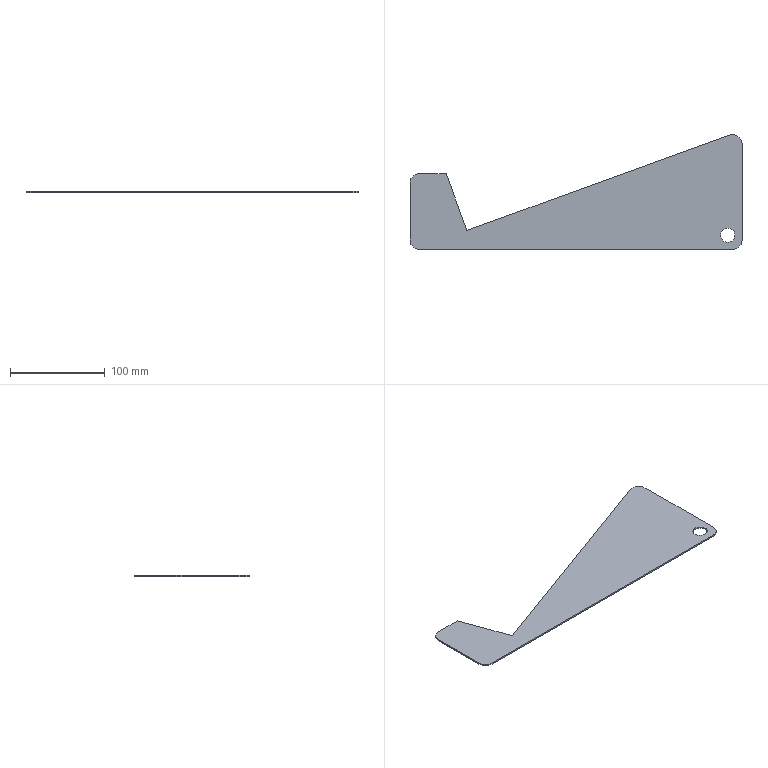Part | SolidWorks | features FlatPattern 1, SMBaseFlange 1, SheetMetal 1 | 1 solid | 14 faces | box 350 x 121.27 x 1.6 mm | volume 39939 mm3 | plane 8 | cylinder 6 | commonest cylinder face diameters 20 x4 15 x2
STEP:
#1=CARTESIAN_POINT('',(633.,10.,1.6));
#2=VERTEX_POINT('',#1);
#3=CARTESIAN_POINT('',(648.,10.,1.6));
#4=VERTEX_POINT('',#3);
#5=CARTESIAN_POINT('',(640.5,10.,1.6));
#6=DIRECTION('',(0.,0.,1.));
#7=DIRECTION('',(1.,0.,0.));
#8=AXIS2_PLACEMENT_3D('',#5,#6,#7);
#9=CIRCLE('',#8,7.5);
#10=EDGE_CURVE('',#2,#4,#9,.T.);
#11=ORIENTED_EDGE('',*,*,#10,.T.);
#12=CARTESIAN_POINT('',(648.,10.,0.));
#13=VERTEX_POINT('',#12);
#14=CARTESIAN_POINT('',(648.,10.,1.6));
#15=DIRECTION('',(0.,0.,-1.));
#16=VECTOR('',#15,1000.);
#17=LINE('',#14,#16);
#18=EDGE_CURVE('',#4,#13,#17,.T.);
#19=ORIENTED_EDGE('',*,*,#18,.T.);
#20=CARTESIAN_POINT('',(633.,10.,0.));
#21=VERTEX_POINT('',#20);
#22=CARTESIAN_POINT('',(640.5,10.,0.));
#23=DIRECTION('',(0.,0.,1.));
#24=DIRECTION('',(1.,0.,0.));
#25=AXIS2_PLACEMENT_3D('',#22,#23,#24);
#26=CIRCLE('',#25,7.5);
#27=EDGE_CURVE('',#21,#13,#26,.T.);
#28=ORIENTED_EDGE('',*,*,#27,.F.);
#29=CARTESIAN_POINT('',(633.,10.,1.6));
#30=DIRECTION('',(0.,0.,-1.));
#31=VECTOR('',#30,1000.);
#32=LINE('',#29,#31);
#33=EDGE_CURVE('',#2,#21,#32,.T.);
#34=ORIENTED_EDGE('',*,*,#33,.F.);
#35=EDGE_LOOP('',(#11,#19,#28,#34));
#36=FACE_OUTER_BOUND('',#35,.T.);
#37=CARTESIAN_POINT('',(640.5,10.,1.6));
#38=DIRECTION('',(0.,0.,-1.));
#39=DIRECTION('',(-1.,0.,0.));
#40=AXIS2_PLACEMENT_3D('',#37,#38,#39);
#41=CYLINDRICAL_SURFACE('',#40,7.5);
#42=ADVANCED_FACE('',(#36),#41,.F.);
#43=CARTESIAN_POINT('',(343.662,75.,1.6));
#44=VERTEX_POINT('',#43);
#45=CARTESIAN_POINT('',(315.5,75.,1.6));
#46=VERTEX_POINT('',#45);
#47=CARTESIAN_POINT('',(343.662,75.,1.6));
#48=DIRECTION('',(-1.,0.,0.));
#49=VECTOR('',#48,1000.);
#50=LINE('',#47,#49);
#51=EDGE_CURVE('',#44,#46,#50,.T.);
#52=ORIENTED_EDGE('',*,*,#51,.T.);
#53=CARTESIAN_POINT('',(305.5,65.,1.6));
#54=VERTEX_POINT('',#53);
#55=CARTESIAN_POINT('',(315.5,65.,1.6));
#56=DIRECTION('',(0.,0.,1.));
#57=DIRECTION('',(1.,0.,0.));
#58=AXIS2_PLACEMENT_3D('',#55,#56,#57);
#59=CIRCLE('',#58,10.);
#60=EDGE_CURVE('',#46,#54,#59,.T.);
#61=ORIENTED_EDGE('',*,*,#60,.T.);
#62=CARTESIAN_POINT('',(305.5,5.,1.6));
#63=VERTEX_POINT('',#62);
#64=CARTESIAN_POINT('',(305.5,5.,1.6));
#65=DIRECTION('',(0.,-1.,0.));
#66=VECTOR('',#65,1000.);
#67=LINE('',#64,#66);
#68=EDGE_CURVE('',#54,#63,#67,.T.);
#69=ORIENTED_EDGE('',*,*,#68,.T.);
#70=CARTESIAN_POINT('',(315.5,-5.,1.6));
#71=VERTEX_POINT('',#70);
#72=CARTESIAN_POINT('',(315.5,5.,1.6));
#73=DIRECTION('',(0.,0.,1.));
#74=DIRECTION('',(-1.,0.,0.));
#75=AXIS2_PLACEMENT_3D('',#72,#73,#74);
#76=CIRCLE('',#75,10.);
#77=EDGE_CURVE('',#63,#71,#76,.T.);
#78=ORIENTED_EDGE('',*,*,#77,.T.);
#79=CARTESIAN_POINT('',(645.5,-5.,1.6));
#80=VERTEX_POINT('',#79);
#81=CARTESIAN_POINT('',(645.5,-5.,1.6));
#82=DIRECTION('',(1.,0.,0.));
#83=VECTOR('',#82,1000.);
#84=LINE('',#81,#83);
#85=EDGE_CURVE('',#71,#80,#84,.T.);
#86=ORIENTED_EDGE('',*,*,#85,.T.);
#87=CARTESIAN_POINT('',(655.5,5.,1.6));
#88=VERTEX_POINT('',#87);
#89=CARTESIAN_POINT('',(645.5,5.,1.6));
#90=DIRECTION('',(0.,0.,1.));
#91=DIRECTION('',(-1.,0.,0.));
#92=AXIS2_PLACEMENT_3D('',#89,#90,#91);
#93=CIRCLE('',#92,10.);
#94=EDGE_CURVE('',#80,#88,#93,.T.);
#95=ORIENTED_EDGE('',*,*,#94,.T.);
#96=CARTESIAN_POINT('',(655.5,106.27,1.6));
#97=VERTEX_POINT('',#96);
#98=CARTESIAN_POINT('',(655.5,106.27,1.6));
#99=DIRECTION('',(0.,1.,0.));
#100=VECTOR('',#99,1000.);
#101=LINE('',#98,#100);
#102=EDGE_CURVE('',#88,#97,#101,.T.);
#103=ORIENTED_EDGE('',*,*,#102,.T.);
#104=CARTESIAN_POINT('',(642.08,115.667,1.6));
#105=VERTEX_POINT('',#104);
#106=CARTESIAN_POINT('',(645.5,106.27,1.6));
#107=DIRECTION('',(0.,0.,1.));
#108=DIRECTION('',(-1.,0.,0.));
#109=AXIS2_PLACEMENT_3D('',#106,#107,#108);
#110=CIRCLE('',#109,10.);
#111=EDGE_CURVE('',#97,#105,#110,.T.);
#112=ORIENTED_EDGE('',*,*,#111,.T.);
#113=CARTESIAN_POINT('',(365.5,15.,1.6));
#114=VERTEX_POINT('',#113);
#115=CARTESIAN_POINT('',(365.5,15.,1.6));
#116=DIRECTION('',(-0.9397,-0.342,0.));
#117=VECTOR('',#116,1000.);
#118=LINE('',#115,#117);
#119=EDGE_CURVE('',#105,#114,#118,.T.);
#120=ORIENTED_EDGE('',*,*,#119,.T.);
#121=CARTESIAN_POINT('',(365.5,15.,1.6));
#122=DIRECTION('',(-0.342,0.9397,0.));
#123=VECTOR('',#122,1000.);
#124=LINE('',#121,#123);
#125=EDGE_CURVE('',#114,#44,#124,.T.);
#126=ORIENTED_EDGE('',*,*,#125,.T.);
#127=EDGE_LOOP('',(#52,#61,#69,#78,#86,#95,#103,#112,#120,#126));
#128=FACE_OUTER_BOUND('',#127,.T.);
#129=ORIENTED_EDGE('',*,*,#10,.F.);
#130=CARTESIAN_POINT('',(640.5,10.,1.6));
#131=DIRECTION('',(0.,0.,1.));
#132=DIRECTION('',(1.,0.,0.));
#133=AXIS2_PLACEMENT_3D('',#130,#131,#132);
#134=CIRCLE('',#133,7.5);
#135=EDGE_CURVE('',#4,#2,#134,.T.);
#136=ORIENTED_EDGE('',*,*,#135,.F.);
#137=EDGE_LOOP('',(#129,#136));
#138=FACE_BOUND('',#137,.T.);
#139=CARTESIAN_POINT('',(315.5,65.,1.6));
#140=DIRECTION('',(0.,0.,1.));
#141=DIRECTION('',(1.,0.,0.));
#142=AXIS2_PLACEMENT_3D('',#139,#140,#141);
#143=PLANE('',#142);
#144=ADVANCED_FACE('',(#128,#138),#143,.T.);
#145=CARTESIAN_POINT('',(343.662,75.,0.));
#146=VERTEX_POINT('',#145);
#147=CARTESIAN_POINT('',(315.5,75.,0.));
#148=VERTEX_POINT('',#147);
#149=CARTESIAN_POINT('',(343.662,75.,0.));
#150=DIRECTION('',(-1.,0.,0.));
#151=VECTOR('',#150,1000.);
#152=LINE('',#149,#151);
#153=EDGE_CURVE('',#146,#148,#152,.T.);
#154=ORIENTED_EDGE('',*,*,#153,.F.);
#155=CARTESIAN_POINT('',(365.5,15.,0.));
#156=VERTEX_POINT('',#155);
#157=CARTESIAN_POINT('',(365.5,15.,0.));
#158=DIRECTION('',(-0.342,0.9397,0.));
#159=VECTOR('',#158,1000.);
#160=LINE('',#157,#159);
#161=EDGE_CURVE('',#156,#146,#160,.T.);
#162=ORIENTED_EDGE('',*,*,#161,.F.);
#163=CARTESIAN_POINT('',(642.08,115.667,0.));
#164=VERTEX_POINT('',#163);
#165=CARTESIAN_POINT('',(365.5,15.,0.));
#166=DIRECTION('',(-0.9397,-0.342,0.));
#167=VECTOR('',#166,1000.);
#168=LINE('',#165,#167);
#169=EDGE_CURVE('',#164,#156,#168,.T.);
#170=ORIENTED_EDGE('',*,*,#169,.F.);
#171=CARTESIAN_POINT('',(655.5,106.27,0.));
#172=VERTEX_POINT('',#171);
#173=CARTESIAN_POINT('',(645.5,106.27,0.));
#174=DIRECTION('',(0.,0.,1.));
#175=DIRECTION('',(-1.,0.,0.));
#176=AXIS2_PLACEMENT_3D('',#173,#174,#175);
#177=CIRCLE('',#176,10.);
#178=EDGE_CURVE('',#172,#164,#177,.T.);
#179=ORIENTED_EDGE('',*,*,#178,.F.);
#180=CARTESIAN_POINT('',(655.5,5.,0.));
#181=VERTEX_POINT('',#180);
#182=CARTESIAN_POINT('',(655.5,106.27,0.));
#183=DIRECTION('',(0.,1.,0.));
#184=VECTOR('',#183,1000.);
#185=LINE('',#182,#184);
#186=EDGE_CURVE('',#181,#172,#185,.T.);
#187=ORIENTED_EDGE('',*,*,#186,.F.);
#188=CARTESIAN_POINT('',(645.5,-5.,0.));
#189=VERTEX_POINT('',#188);
#190=CARTESIAN_POINT('',(645.5,5.,0.));
#191=DIRECTION('',(0.,0.,1.));
#192=DIRECTION('',(-1.,0.,0.));
#193=AXIS2_PLACEMENT_3D('',#190,#191,#192);
#194=CIRCLE('',#193,10.);
#195=EDGE_CURVE('',#189,#181,#194,.T.);
#196=ORIENTED_EDGE('',*,*,#195,.F.);
#197=CARTESIAN_POINT('',(315.5,-5.,0.));
#198=VERTEX_POINT('',#197);
#199=CARTESIAN_POINT('',(645.5,-5.,0.));
#200=DIRECTION('',(1.,0.,0.));
#201=VECTOR('',#200,1000.);
#202=LINE('',#199,#201);
#203=EDGE_CURVE('',#198,#189,#202,.T.);
#204=ORIENTED_EDGE('',*,*,#203,.F.);
#205=CARTESIAN_POINT('',(305.5,5.,0.));
#206=VERTEX_POINT('',#205);
#207=CARTESIAN_POINT('',(315.5,5.,0.));
#208=DIRECTION('',(0.,0.,1.));
#209=DIRECTION('',(-1.,0.,0.));
#210=AXIS2_PLACEMENT_3D('',#207,#208,#209);
#211=CIRCLE('',#210,10.);
#212=EDGE_CURVE('',#206,#198,#211,.T.);
#213=ORIENTED_EDGE('',*,*,#212,.F.);
#214=CARTESIAN_POINT('',(305.5,65.,0.));
#215=VERTEX_POINT('',#214);
#216=CARTESIAN_POINT('',(305.5,5.,0.));
#217=DIRECTION('',(0.,-1.,0.));
#218=VECTOR('',#217,1000.);
#219=LINE('',#216,#218);
#220=EDGE_CURVE('',#215,#206,#219,.T.);
#221=ORIENTED_EDGE('',*,*,#220,.F.);
#222=CARTESIAN_POINT('',(315.5,65.,0.));
#223=DIRECTION('',(0.,0.,1.));
#224=DIRECTION('',(1.,0.,0.));
#225=AXIS2_PLACEMENT_3D('',#222,#223,#224);
#226=CIRCLE('',#225,10.);
#227=EDGE_CURVE('',#148,#215,#226,.T.);
#228=ORIENTED_EDGE('',*,*,#227,.F.);
#229=EDGE_LOOP('',(#154,#162,#170,#179,#187,#196,#204,#213,#221,#228));
#230=FACE_OUTER_BOUND('',#229,.T.);
#231=ORIENTED_EDGE('',*,*,#27,.T.);
#232=CARTESIAN_POINT('',(640.5,10.,0.));
#233=DIRECTION('',(0.,0.,1.));
#234=DIRECTION('',(1.,0.,0.));
#235=AXIS2_PLACEMENT_3D('',#232,#233,#234);
#236=CIRCLE('',#235,7.5);
#237=EDGE_CURVE('',#13,#21,#236,.T.);
#238=ORIENTED_EDGE('',*,*,#237,.T.);
#239=EDGE_LOOP('',(#231,#238));
#240=FACE_BOUND('',#239,.T.);
#241=CARTESIAN_POINT('',(315.5,65.,0.));
#242=DIRECTION('',(0.,0.,1.));
#243=DIRECTION('',(1.,0.,0.));
#244=AXIS2_PLACEMENT_3D('',#241,#242,#243);
#245=PLANE('',#244);
#246=ADVANCED_FACE('',(#230,#240),#245,.F.);
#247=ORIENTED_EDGE('',*,*,#153,.T.);
#248=CARTESIAN_POINT('',(315.5,75.,1.6));
#249=DIRECTION('',(0.,0.,-1.));
#250=VECTOR('',#249,1000.);
#251=LINE('',#248,#250);
#252=EDGE_CURVE('',#46,#148,#251,.T.);
#253=ORIENTED_EDGE('',*,*,#252,.F.);
#254=ORIENTED_EDGE('',*,*,#51,.F.);
#255=CARTESIAN_POINT('',(343.662,75.,1.6));
#256=DIRECTION('',(0.,0.,-1.));
#257=VECTOR('',#256,1000.);
#258=LINE('',#255,#257);
#259=EDGE_CURVE('',#44,#146,#258,.T.);
#260=ORIENTED_EDGE('',*,*,#259,.T.);
#261=EDGE_LOOP('',(#247,#253,#254,#260));
#262=FACE_OUTER_BOUND('',#261,.T.);
#263=CARTESIAN_POINT('',(343.662,75.,1.6));
#264=DIRECTION('',(0.,-1.,0.));
#265=DIRECTION('',(0.,0.,-1.));
#266=AXIS2_PLACEMENT_3D('',#263,#264,#265);
#267=PLANE('',#266);
#268=ADVANCED_FACE('',(#262),#267,.F.);
#269=ORIENTED_EDGE('',*,*,#227,.T.);
#270=CARTESIAN_POINT('',(305.5,65.,1.6));
#271=DIRECTION('',(0.,0.,-1.));
#272=VECTOR('',#271,1000.);
#273=LINE('',#270,#272);
#274=EDGE_CURVE('',#54,#215,#273,.T.);
#275=ORIENTED_EDGE('',*,*,#274,.F.);
#276=ORIENTED_EDGE('',*,*,#60,.F.);
#277=ORIENTED_EDGE('',*,*,#252,.T.);
#278=EDGE_LOOP('',(#269,#275,#276,#277));
#279=FACE_OUTER_BOUND('',#278,.T.);
#280=CARTESIAN_POINT('',(315.5,65.,1.6));
#281=DIRECTION('',(0.,0.,-1.));
#282=DIRECTION('',(-1.,0.,0.));
#283=AXIS2_PLACEMENT_3D('',#280,#281,#282);
#284=CYLINDRICAL_SURFACE('',#283,10.);
#285=ADVANCED_FACE('',(#279),#284,.T.);
#286=ORIENTED_EDGE('',*,*,#220,.T.);
#287=CARTESIAN_POINT('',(305.5,5.,1.6));
#288=DIRECTION('',(0.,0.,-1.));
#289=VECTOR('',#288,1000.);
#290=LINE('',#287,#289);
#291=EDGE_CURVE('',#63,#206,#290,.T.);
#292=ORIENTED_EDGE('',*,*,#291,.F.);
#293=ORIENTED_EDGE('',*,*,#68,.F.);
#294=ORIENTED_EDGE('',*,*,#274,.T.);
#295=EDGE_LOOP('',(#286,#292,#293,#294));
#296=FACE_OUTER_BOUND('',#295,.T.);
#297=CARTESIAN_POINT('',(305.5,5.,1.6));
#298=DIRECTION('',(1.,0.,0.));
#299=DIRECTION('',(0.,0.,-1.));
#300=AXIS2_PLACEMENT_3D('',#297,#298,#299);
#301=PLANE('',#300);
#302=ADVANCED_FACE('',(#296),#301,.F.);
#303=ORIENTED_EDGE('',*,*,#212,.T.);
#304=CARTESIAN_POINT('',(315.5,-5.,1.6));
#305=DIRECTION('',(0.,0.,-1.));
#306=VECTOR('',#305,1000.);
#307=LINE('',#304,#306);
#308=EDGE_CURVE('',#71,#198,#307,.T.);
#309=ORIENTED_EDGE('',*,*,#308,.F.);
#310=ORIENTED_EDGE('',*,*,#77,.F.);
#311=ORIENTED_EDGE('',*,*,#291,.T.);
#312=EDGE_LOOP('',(#303,#309,#310,#311));
#313=FACE_OUTER_BOUND('',#312,.T.);
#314=CARTESIAN_POINT('',(315.5,5.,1.6));
#315=DIRECTION('',(0.,0.,-1.));
#316=DIRECTION('',(-1.,0.,0.));
#317=AXIS2_PLACEMENT_3D('',#314,#315,#316);
#318=CYLINDRICAL_SURFACE('',#317,10.);
#319=ADVANCED_FACE('',(#313),#318,.T.);
#320=ORIENTED_EDGE('',*,*,#203,.T.);
#321=CARTESIAN_POINT('',(645.5,-5.,1.6));
#322=DIRECTION('',(0.,0.,-1.));
#323=VECTOR('',#322,1000.);
#324=LINE('',#321,#323);
#325=EDGE_CURVE('',#80,#189,#324,.T.);
#326=ORIENTED_EDGE('',*,*,#325,.F.);
#327=ORIENTED_EDGE('',*,*,#85,.F.);
#328=ORIENTED_EDGE('',*,*,#308,.T.);
#329=EDGE_LOOP('',(#320,#326,#327,#328));
#330=FACE_OUTER_BOUND('',#329,.T.);
#331=CARTESIAN_POINT('',(645.5,-5.,1.6));
#332=DIRECTION('',(0.,1.,0.));
#333=DIRECTION('',(0.,0.,1.));
#334=AXIS2_PLACEMENT_3D('',#331,#332,#333);
#335=PLANE('',#334);
#336=ADVANCED_FACE('',(#330),#335,.F.);
#337=ORIENTED_EDGE('',*,*,#195,.T.);
#338=CARTESIAN_POINT('',(655.5,5.,1.6));
#339=DIRECTION('',(0.,0.,-1.));
#340=VECTOR('',#339,1000.);
#341=LINE('',#338,#340);
#342=EDGE_CURVE('',#88,#181,#341,.T.);
#343=ORIENTED_EDGE('',*,*,#342,.F.);
#344=ORIENTED_EDGE('',*,*,#94,.F.);
#345=ORIENTED_EDGE('',*,*,#325,.T.);
#346=EDGE_LOOP('',(#337,#343,#344,#345));
#347=FACE_OUTER_BOUND('',#346,.T.);
#348=CARTESIAN_POINT('',(645.5,5.,1.6));
#349=DIRECTION('',(0.,0.,-1.));
#350=DIRECTION('',(-1.,0.,0.));
#351=AXIS2_PLACEMENT_3D('',#348,#349,#350);
#352=CYLINDRICAL_SURFACE('',#351,10.);
#353=ADVANCED_FACE('',(#347),#352,.T.);
#354=ORIENTED_EDGE('',*,*,#186,.T.);
#355=CARTESIAN_POINT('',(655.5,106.27,1.6));
#356=DIRECTION('',(0.,0.,-1.));
#357=VECTOR('',#356,1000.);
#358=LINE('',#355,#357);
#359=EDGE_CURVE('',#97,#172,#358,.T.);
#360=ORIENTED_EDGE('',*,*,#359,.F.);
#361=ORIENTED_EDGE('',*,*,#102,.F.);
#362=ORIENTED_EDGE('',*,*,#342,.T.);
#363=EDGE_LOOP('',(#354,#360,#361,#362));
#364=FACE_OUTER_BOUND('',#363,.T.);
#365=CARTESIAN_POINT('',(655.5,106.27,1.6));
#366=DIRECTION('',(-1.,0.,0.));
#367=DIRECTION('',(0.,0.,1.));
#368=AXIS2_PLACEMENT_3D('',#365,#366,#367);
#369=PLANE('',#368);
#370=ADVANCED_FACE('',(#364),#369,.F.);
#371=ORIENTED_EDGE('',*,*,#178,.T.);
#372=CARTESIAN_POINT('',(642.08,115.667,1.6));
#373=DIRECTION('',(0.,0.,-1.));
#374=VECTOR('',#373,1000.);
#375=LINE('',#372,#374);
#376=EDGE_CURVE('',#105,#164,#375,.T.);
#377=ORIENTED_EDGE('',*,*,#376,.F.);
#378=ORIENTED_EDGE('',*,*,#111,.F.);
#379=ORIENTED_EDGE('',*,*,#359,.T.);
#380=EDGE_LOOP('',(#371,#377,#378,#379));
#381=FACE_OUTER_BOUND('',#380,.T.);
#382=CARTESIAN_POINT('',(645.5,106.27,1.6));
#383=DIRECTION('',(0.,0.,-1.));
#384=DIRECTION('',(-1.,0.,0.));
#385=AXIS2_PLACEMENT_3D('',#382,#383,#384);
#386=CYLINDRICAL_SURFACE('',#385,10.);
#387=ADVANCED_FACE('',(#381),#386,.T.);
#388=ORIENTED_EDGE('',*,*,#169,.T.);
#389=CARTESIAN_POINT('',(365.5,15.,1.6));
#390=DIRECTION('',(0.,0.,-1.));
#391=VECTOR('',#390,1000.);
#392=LINE('',#389,#391);
#393=EDGE_CURVE('',#114,#156,#392,.T.);
#394=ORIENTED_EDGE('',*,*,#393,.F.);
#395=ORIENTED_EDGE('',*,*,#119,.F.);
#396=ORIENTED_EDGE('',*,*,#376,.T.);
#397=EDGE_LOOP('',(#388,#394,#395,#396));
#398=FACE_OUTER_BOUND('',#397,.T.);
#399=CARTESIAN_POINT('',(365.5,15.,1.6));
#400=DIRECTION('',(0.342,-0.9397,0.));
#401=DIRECTION('',(0.9397,0.342,0.));
#402=AXIS2_PLACEMENT_3D('',#399,#400,#401);
#403=PLANE('',#402);
#404=ADVANCED_FACE('',(#398),#403,.F.);
#405=ORIENTED_EDGE('',*,*,#161,.T.);
#406=ORIENTED_EDGE('',*,*,#259,.F.);
#407=ORIENTED_EDGE('',*,*,#125,.F.);
#408=ORIENTED_EDGE('',*,*,#393,.T.);
#409=EDGE_LOOP('',(#405,#406,#407,#408));
#410=FACE_OUTER_BOUND('',#409,.T.);
#411=CARTESIAN_POINT('',(365.5,15.,1.6));
#412=DIRECTION('',(-0.9397,-0.342,0.));
#413=DIRECTION('',(0.342,-0.9397,0.));
#414=AXIS2_PLACEMENT_3D('',#411,#412,#413);
#415=PLANE('',#414);
#416=ADVANCED_FACE('',(#410),#415,.F.);
#417=ORIENTED_EDGE('',*,*,#18,.F.);
#418=ORIENTED_EDGE('',*,*,#135,.T.);
#419=ORIENTED_EDGE('',*,*,#33,.T.);
#420=ORIENTED_EDGE('',*,*,#237,.F.);
#421=EDGE_LOOP('',(#417,#418,#419,#420));
#422=FACE_OUTER_BOUND('',#421,.T.);
#423=CARTESIAN_POINT('',(640.5,10.,1.6));
#424=DIRECTION('',(0.,0.,-1.));
#425=DIRECTION('',(-1.,0.,0.));
#426=AXIS2_PLACEMENT_3D('',#423,#424,#425);
#427=CYLINDRICAL_SURFACE('',#426,7.5);
#428=ADVANCED_FACE('',(#422),#427,.F.);
#429=CLOSED_SHELL('',(#42,#144,#246,#268,#285,#302,#319,#336,#353,#370,#387,#404,#416,#428));
#430=MANIFOLD_SOLID_BREP('',#429);
#431=CARTESIAN_POINT('',(0.,0.,0.));
#432=DIRECTION('',(0.,0.,1.));
#433=DIRECTION('',(1.,0.,0.));
#434=AXIS2_PLACEMENT_3D('',#431,#432,#433);
#435=(LENGTH_UNIT()NAMED_UNIT(*)SI_UNIT(.MILLI.,.METRE.));
#436=UNCERTAINTY_MEASURE_WITH_UNIT(LENGTH_MEASURE(0.00001),#435,'','');
#437=(NAMED_UNIT(*)PLANE_ANGLE_UNIT()SI_UNIT($,.RADIAN.));
#438=(NAMED_UNIT(*)SI_UNIT($,.STERADIAN.)SOLID_ANGLE_UNIT());
#439=(GEOMETRIC_REPRESENTATION_CONTEXT(3)GLOBAL_UNCERTAINTY_ASSIGNED_CONTEXT((#436))GLOBAL_UNIT_ASSIGNED_CONTEXT((#435,#437,#438))REPRESENTATION_CONTEXT('',''));
#440=ADVANCED_BREP_SHAPE_REPRESENTATION('',(#430,#434),#439);